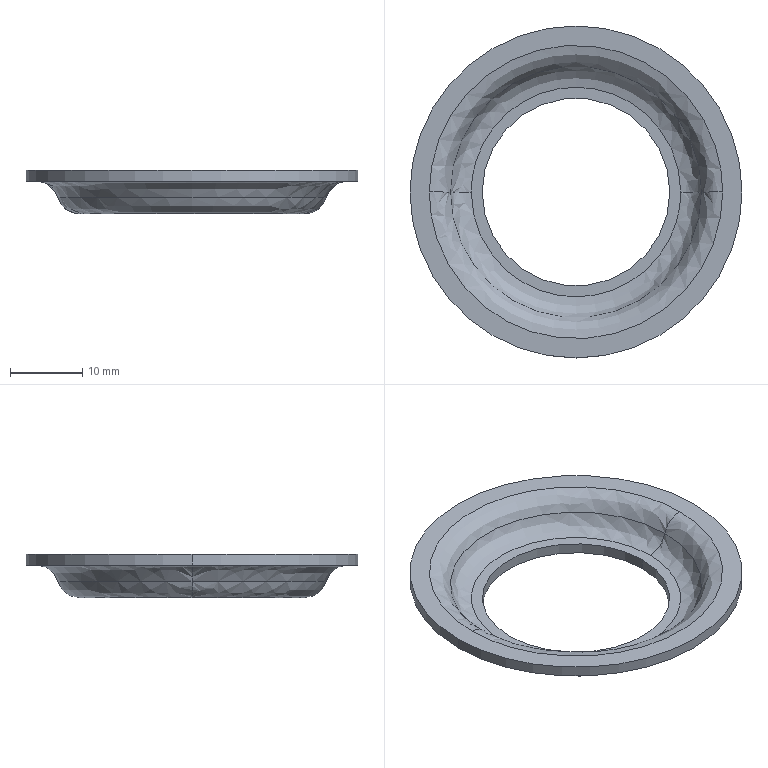Part | SolidWorks | features BaseBody 1 | 1 solid | 16 faces | box 46 x 46 x 6 mm | volume 2288 mm3 | spline 8 | cylinder 4 | plane 4 | commonest cylinder face diameters 26 x2 46 x2